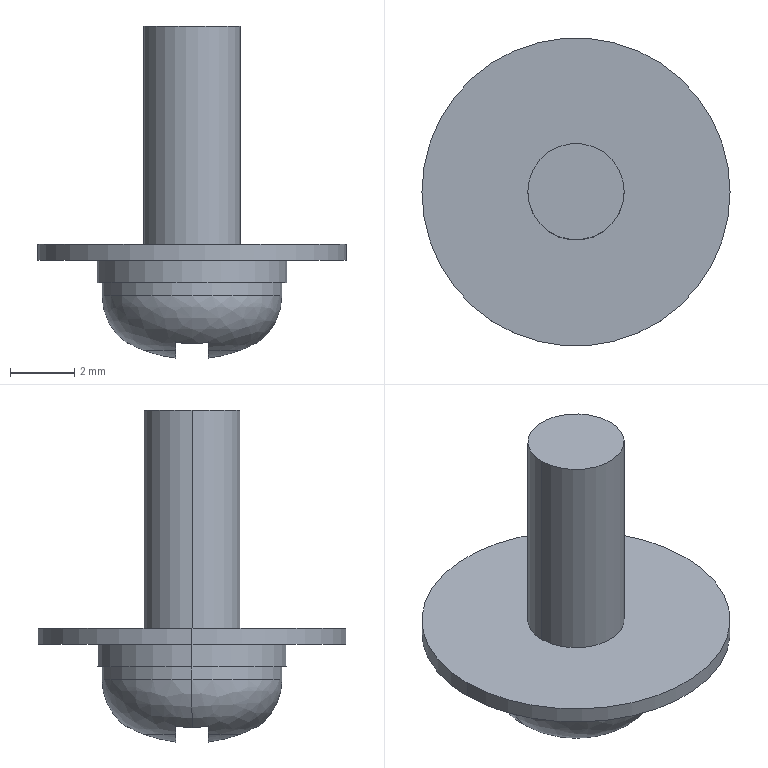Part | SolidWorks | 1 solid | 31 faces | box 9.6 x 9.6 x 10.343 mm | volume 135.072 mm3 | plane 17 | cylinder 8 | spline 6 | commonest cylinder face diameters 3 x2 5.6 x2 5.9 x2 9.6 x2
STEP:
#1=CARTESIAN_POINT('',(0.5,0.5,-1.6));
#2=VERTEX_POINT('',#1);
#3=CARTESIAN_POINT('',(0.5,2.,-1.6));
#4=VERTEX_POINT('',#3);
#5=CARTESIAN_POINT('',(0.5,2.,-1.6));
#6=DIRECTION('',(0.,1.,0.));
#7=VECTOR('',#6,1000.);
#8=LINE('',#5,#7);
#9=EDGE_CURVE('',#2,#4,#8,.T.);
#10=ORIENTED_EDGE('',*,*,#9,.T.);
#11=CARTESIAN_POINT('',(0.5,2.,-3.057));
#12=VERTEX_POINT('',#11);
#13=CARTESIAN_POINT('',(0.5,2.,-1.6));
#14=DIRECTION('',(0.,0.,-1.));
#15=VECTOR('',#14,1000.);
#16=LINE('',#13,#15);
#17=EDGE_CURVE('',#4,#12,#16,.T.);
#18=ORIENTED_EDGE('',*,*,#17,.T.);
#19=CARTESIAN_POINT('',(0.5,1.52,-3.3));
#20=VERTEX_POINT('',#19);
#21=CARTESIAN_POINT('',(0.5,2.,-3.057));
#22=CARTESIAN_POINT('',(0.5,1.853,-3.161));
#23=CARTESIAN_POINT('',(0.5,1.693,-3.242));
#24=CARTESIAN_POINT('',(0.5,1.52,-3.3));
#25=B_SPLINE_CURVE_WITH_KNOTS('',3,(#21,#22,#23,#24),.UNSPECIFIED.,.F.,.F.,(4,4),(0.,1.),.UNSPECIFIED.);
#26=EDGE_CURVE('',#12,#20,#25,.T.);
#27=ORIENTED_EDGE('',*,*,#26,.T.);
#28=CARTESIAN_POINT('',(0.5,0.5,-3.543));
#29=VERTEX_POINT('',#28);
#30=CARTESIAN_POINT('',(0.5,1.52,-3.3));
#31=CARTESIAN_POINT('',(0.5,1.19,-3.422));
#32=CARTESIAN_POINT('',(0.5,0.8497,-3.503));
#33=CARTESIAN_POINT('',(0.5,0.5,-3.543));
#34=B_SPLINE_CURVE_WITH_KNOTS('',3,(#30,#31,#32,#33),.UNSPECIFIED.,.F.,.F.,(4,4),(0.,1.),.UNSPECIFIED.);
#35=EDGE_CURVE('',#20,#29,#34,.T.);
#36=ORIENTED_EDGE('',*,*,#35,.T.);
#37=CARTESIAN_POINT('',(0.5,0.5,-1.6));
#38=DIRECTION('',(0.,0.,-1.));
#39=VECTOR('',#38,1000.);
#40=LINE('',#37,#39);
#41=EDGE_CURVE('',#2,#29,#40,.T.);
#42=ORIENTED_EDGE('',*,*,#41,.F.);
#43=EDGE_LOOP('',(#10,#18,#27,#36,#42));
#44=FACE_OUTER_BOUND('',#43,.T.);
#45=CARTESIAN_POINT('',(0.5,2.,-1.6));
#46=DIRECTION('',(-1.,0.,0.));
#47=DIRECTION('',(0.,0.,1.));
#48=AXIS2_PLACEMENT_3D('',#45,#46,#47);
#49=PLANE('',#48);
#50=ADVANCED_FACE('',(#44),#49,.T.);
#51=ORIENTED_EDGE('',*,*,#41,.T.);
#52=CARTESIAN_POINT('',(1.52,0.5,-3.3));
#53=VERTEX_POINT('',#52);
#54=CARTESIAN_POINT('',(0.,0.5,0.8167));
#55=DIRECTION('',(0.,-1.,0.));
#56=DIRECTION('',(0.,0.,1.));
#57=AXIS2_PLACEMENT_3D('',#54,#55,#56);
#58=CIRCLE('',#57,4.388);
#59=EDGE_CURVE('',#29,#53,#58,.T.);
#60=ORIENTED_EDGE('',*,*,#59,.T.);
#61=CARTESIAN_POINT('',(2.,0.5,-3.057));
#62=VERTEX_POINT('',#61);
#63=CARTESIAN_POINT('',(1.52,0.5,-3.3));
#64=CARTESIAN_POINT('',(1.691,0.5,-3.243));
#65=CARTESIAN_POINT('',(1.853,0.5,-3.161));
#66=CARTESIAN_POINT('',(2.,0.5,-3.057));
#67=B_SPLINE_CURVE_WITH_KNOTS('',3,(#63,#64,#65,#66),.UNSPECIFIED.,.F.,.F.,(4,4),(0.,0.0005389),.UNSPECIFIED.);
#68=EDGE_CURVE('',#53,#62,#67,.T.);
#69=ORIENTED_EDGE('',*,*,#68,.T.);
#70=CARTESIAN_POINT('',(2.,0.5,-1.6));
#71=VERTEX_POINT('',#70);
#72=CARTESIAN_POINT('',(2.,0.5,-1.6));
#73=DIRECTION('',(0.,0.,-1.));
#74=VECTOR('',#73,1000.);
#75=LINE('',#72,#74);
#76=EDGE_CURVE('',#71,#62,#75,.T.);
#77=ORIENTED_EDGE('',*,*,#76,.F.);
#78=CARTESIAN_POINT('',(0.5,0.5,-1.6));
#79=DIRECTION('',(-1.,0.,0.));
#80=VECTOR('',#79,1000.);
#81=LINE('',#78,#80);
#82=EDGE_CURVE('',#71,#2,#81,.T.);
#83=ORIENTED_EDGE('',*,*,#82,.T.);
#84=EDGE_LOOP('',(#51,#60,#69,#77,#83));
#85=FACE_OUTER_BOUND('',#84,.T.);
#86=CARTESIAN_POINT('',(0.5,0.5,-1.6));
#87=DIRECTION('',(0.,-1.,0.));
#88=DIRECTION('',(0.,0.,-1.));
#89=AXIS2_PLACEMENT_3D('',#86,#87,#88);
#90=PLANE('',#89);
#91=ADVANCED_FACE('',(#85),#90,.T.);
#92=CARTESIAN_POINT('',(0.5,-0.5,-1.6));
#93=VERTEX_POINT('',#92);
#94=CARTESIAN_POINT('',(2.,-0.5,-1.6));
#95=VERTEX_POINT('',#94);
#96=CARTESIAN_POINT('',(2.,-0.5,-1.6));
#97=DIRECTION('',(1.,0.,0.));
#98=VECTOR('',#97,1000.);
#99=LINE('',#96,#98);
#100=EDGE_CURVE('',#93,#95,#99,.T.);
#101=ORIENTED_EDGE('',*,*,#100,.T.);
#102=CARTESIAN_POINT('',(2.,-0.5,-3.057));
#103=VERTEX_POINT('',#102);
#104=CARTESIAN_POINT('',(2.,-0.5,-1.6));
#105=DIRECTION('',(0.,0.,1.));
#106=VECTOR('',#105,1000.);
#107=LINE('',#104,#106);
#108=EDGE_CURVE('',#103,#95,#107,.T.);
#109=ORIENTED_EDGE('',*,*,#108,.F.);
#110=CARTESIAN_POINT('',(1.52,-0.5,-3.3));
#111=VERTEX_POINT('',#110);
#112=CARTESIAN_POINT('',(2.,-0.5,-3.057));
#113=CARTESIAN_POINT('',(1.853,-0.5,-3.161));
#114=CARTESIAN_POINT('',(1.693,-0.5,-3.242));
#115=CARTESIAN_POINT('',(1.52,-0.5,-3.3));
#116=B_SPLINE_CURVE_WITH_KNOTS('',3,(#112,#113,#114,#115),.UNSPECIFIED.,.F.,.F.,(4,4),(0.,1.),.UNSPECIFIED.);
#117=EDGE_CURVE('',#103,#111,#116,.T.);
#118=ORIENTED_EDGE('',*,*,#117,.T.);
#119=CARTESIAN_POINT('',(0.5,-0.5,-3.543));
#120=VERTEX_POINT('',#119);
#121=CARTESIAN_POINT('',(0.,-0.5,0.8167));
#122=DIRECTION('',(0.,1.,0.));
#123=DIRECTION('',(0.,0.,1.));
#124=AXIS2_PLACEMENT_3D('',#121,#122,#123);
#125=CIRCLE('',#124,4.388);
#126=EDGE_CURVE('',#111,#120,#125,.T.);
#127=ORIENTED_EDGE('',*,*,#126,.T.);
#128=CARTESIAN_POINT('',(0.5,-0.5,-1.6));
#129=DIRECTION('',(0.,0.,-1.));
#130=VECTOR('',#129,1000.);
#131=LINE('',#128,#130);
#132=EDGE_CURVE('',#93,#120,#131,.T.);
#133=ORIENTED_EDGE('',*,*,#132,.F.);
#134=EDGE_LOOP('',(#101,#109,#118,#127,#133));
#135=FACE_OUTER_BOUND('',#134,.T.);
#136=CARTESIAN_POINT('',(2.,-0.5,-1.6));
#137=DIRECTION('',(0.,1.,0.));
#138=DIRECTION('',(1.,0.,0.));
#139=AXIS2_PLACEMENT_3D('',#136,#137,#138);
#140=PLANE('',#139);
#141=ADVANCED_FACE('',(#135),#140,.T.);
#142=CARTESIAN_POINT('',(-0.5,-0.5,-1.6));
#143=VERTEX_POINT('',#142);
#144=CARTESIAN_POINT('',(-0.5,-2.,-1.6));
#145=VERTEX_POINT('',#144);
#146=CARTESIAN_POINT('',(-0.5,-2.,-1.6));
#147=DIRECTION('',(0.,-1.,0.));
#148=VECTOR('',#147,1000.);
#149=LINE('',#146,#148);
#150=EDGE_CURVE('',#143,#145,#149,.T.);
#151=ORIENTED_EDGE('',*,*,#150,.T.);
#152=CARTESIAN_POINT('',(-0.5,-2.,-3.057));
#153=VERTEX_POINT('',#152);
#154=CARTESIAN_POINT('',(-0.5,-2.,-1.6));
#155=DIRECTION('',(0.,0.,-1.));
#156=VECTOR('',#155,1000.);
#157=LINE('',#154,#156);
#158=EDGE_CURVE('',#145,#153,#157,.T.);
#159=ORIENTED_EDGE('',*,*,#158,.T.);
#160=CARTESIAN_POINT('',(-0.5,-1.52,-3.3));
#161=VERTEX_POINT('',#160);
#162=CARTESIAN_POINT('',(-0.5,-2.,-3.057));
#163=CARTESIAN_POINT('',(-0.5,-1.853,-3.161));
#164=CARTESIAN_POINT('',(-0.5,-1.693,-3.242));
#165=CARTESIAN_POINT('',(-0.5,-1.52,-3.3));
#166=B_SPLINE_CURVE_WITH_KNOTS('',3,(#162,#163,#164,#165),.UNSPECIFIED.,.F.,.F.,(4,4),(0.,1.),.UNSPECIFIED.);
#167=EDGE_CURVE('',#153,#161,#166,.T.);
#168=ORIENTED_EDGE('',*,*,#167,.T.);
#169=CARTESIAN_POINT('',(-0.5,-0.5,-3.543));
#170=VERTEX_POINT('',#169);
#171=CARTESIAN_POINT('',(-0.5,-1.52,-3.3));
#172=CARTESIAN_POINT('',(-0.5,-1.19,-3.422));
#173=CARTESIAN_POINT('',(-0.5,-0.8497,-3.503));
#174=CARTESIAN_POINT('',(-0.5,-0.5,-3.543));
#175=B_SPLINE_CURVE_WITH_KNOTS('',3,(#171,#172,#173,#174),.UNSPECIFIED.,.F.,.F.,(4,4),(0.,1.),.UNSPECIFIED.);
#176=EDGE_CURVE('',#161,#170,#175,.T.);
#177=ORIENTED_EDGE('',*,*,#176,.T.);
#178=CARTESIAN_POINT('',(-0.5,-0.5,-1.6));
#179=DIRECTION('',(0.,0.,-1.));
#180=VECTOR('',#179,1000.);
#181=LINE('',#178,#180);
#182=EDGE_CURVE('',#143,#170,#181,.T.);
#183=ORIENTED_EDGE('',*,*,#182,.F.);
#184=EDGE_LOOP('',(#151,#159,#168,#177,#183));
#185=FACE_OUTER_BOUND('',#184,.T.);
#186=CARTESIAN_POINT('',(-0.5,-2.,-1.6));
#187=DIRECTION('',(1.,0.,0.));
#188=DIRECTION('',(0.,1.,0.));
#189=AXIS2_PLACEMENT_3D('',#186,#187,#188);
#190=PLANE('',#189);
#191=ADVANCED_FACE('',(#185),#190,.T.);
#192=CARTESIAN_POINT('',(2.,2.,-1.6));
#193=DIRECTION('',(0.,-1.,0.));
#194=VECTOR('',#193,1000.);
#195=LINE('',#192,#194);
#196=EDGE_CURVE('',#71,#95,#195,.T.);
#197=ORIENTED_EDGE('',*,*,#196,.F.);
#198=ORIENTED_EDGE('',*,*,#76,.T.);
#199=CARTESIAN_POINT('',(2.,0.,-3.1));
#200=VERTEX_POINT('',#199);
#201=CARTESIAN_POINT('',(2.,0.5,-3.057));
#202=CARTESIAN_POINT('',(2.,0.3381,-3.085));
#203=CARTESIAN_POINT('',(2.,0.1714,-3.1));
#204=CARTESIAN_POINT('',(2.,0.,-3.1));
#205=B_SPLINE_CURVE_WITH_KNOTS('',3,(#201,#202,#203,#204),.UNSPECIFIED.,.F.,.F.,(4,4),(0.,1.),.UNSPECIFIED.);
#206=EDGE_CURVE('',#62,#200,#205,.T.);
#207=ORIENTED_EDGE('',*,*,#206,.T.);
#208=CARTESIAN_POINT('',(2.,0.,-3.1));
#209=CARTESIAN_POINT('',(2.,-0.1714,-3.1));
#210=CARTESIAN_POINT('',(2.,-0.3381,-3.085));
#211=CARTESIAN_POINT('',(2.,-0.5,-3.057));
#212=B_SPLINE_CURVE_WITH_KNOTS('',3,(#208,#209,#210,#211),.UNSPECIFIED.,.F.,.F.,(4,4),(0.,1.),.UNSPECIFIED.);
#213=EDGE_CURVE('',#200,#103,#212,.T.);
#214=ORIENTED_EDGE('',*,*,#213,.T.);
#215=ORIENTED_EDGE('',*,*,#108,.T.);
#216=EDGE_LOOP('',(#197,#198,#207,#214,#215));
#217=FACE_OUTER_BOUND('',#216,.T.);
#218=CARTESIAN_POINT('',(2.,0.5,-1.6));
#219=DIRECTION('',(-1.,0.,0.));
#220=DIRECTION('',(0.,0.,1.));
#221=AXIS2_PLACEMENT_3D('',#218,#219,#220);
#222=PLANE('',#221);
#223=ADVANCED_FACE('',(#217),#222,.T.);
#224=ORIENTED_EDGE('',*,*,#132,.T.);
#225=CARTESIAN_POINT('',(0.5,-1.52,-3.3));
#226=VERTEX_POINT('',#225);
#227=CARTESIAN_POINT('',(0.5,-0.5,-3.543));
#228=CARTESIAN_POINT('',(0.5,-0.8497,-3.503));
#229=CARTESIAN_POINT('',(0.5,-1.19,-3.422));
#230=CARTESIAN_POINT('',(0.5,-1.52,-3.3));
#231=B_SPLINE_CURVE_WITH_KNOTS('',3,(#227,#228,#229,#230),.UNSPECIFIED.,.F.,.F.,(4,4),(0.,1.),.UNSPECIFIED.);
#232=EDGE_CURVE('',#120,#226,#231,.T.);
#233=ORIENTED_EDGE('',*,*,#232,.T.);
#234=CARTESIAN_POINT('',(0.5,-2.,-3.057));
#235=VERTEX_POINT('',#234);
#236=CARTESIAN_POINT('',(0.5,-1.52,-3.3));
#237=CARTESIAN_POINT('',(0.5,-1.691,-3.243));
#238=CARTESIAN_POINT('',(0.5,-1.853,-3.161));
#239=CARTESIAN_POINT('',(0.5,-2.,-3.057));
#240=B_SPLINE_CURVE_WITH_KNOTS('',3,(#236,#237,#238,#239),.UNSPECIFIED.,.F.,.F.,(4,4),(0.,0.0005389),.UNSPECIFIED.);
#241=EDGE_CURVE('',#226,#235,#240,.T.);
#242=ORIENTED_EDGE('',*,*,#241,.T.);
#243=CARTESIAN_POINT('',(0.5,-2.,-1.6));
#244=VERTEX_POINT('',#243);
#245=CARTESIAN_POINT('',(0.5,-2.,-1.6));
#246=DIRECTION('',(0.,0.,1.));
#247=VECTOR('',#246,1000.);
#248=LINE('',#245,#247);
#249=EDGE_CURVE('',#235,#244,#248,.T.);
#250=ORIENTED_EDGE('',*,*,#249,.T.);
#251=CARTESIAN_POINT('',(0.5,2.,-1.6));
#252=DIRECTION('',(0.,-1.,0.));
#253=VECTOR('',#252,1000.);
#254=LINE('',#251,#253);
#255=EDGE_CURVE('',#93,#244,#254,.T.);
#256=ORIENTED_EDGE('',*,*,#255,.F.);
#257=EDGE_LOOP('',(#224,#233,#242,#250,#256));
#258=FACE_OUTER_BOUND('',#257,.T.);
#259=CARTESIAN_POINT('',(0.5,-0.5,-1.6));
#260=DIRECTION('',(-1.,0.,0.));
#261=DIRECTION('',(0.,0.,1.));
#262=AXIS2_PLACEMENT_3D('',#259,#260,#261);
#263=PLANE('',#262);
#264=ADVANCED_FACE('',(#258),#263,.T.);
#265=ORIENTED_EDGE('',*,*,#182,.T.);
#266=CARTESIAN_POINT('',(-1.52,-0.5,-3.3));
#267=VERTEX_POINT('',#266);
#268=CARTESIAN_POINT('',(0.,-0.5,0.8167));
#269=DIRECTION('',(0.,1.,0.));
#270=DIRECTION('',(0.,0.,1.));
#271=AXIS2_PLACEMENT_3D('',#268,#269,#270);
#272=CIRCLE('',#271,4.388);
#273=EDGE_CURVE('',#170,#267,#272,.T.);
#274=ORIENTED_EDGE('',*,*,#273,.T.);
#275=CARTESIAN_POINT('',(-2.,-0.5,-3.057));
#276=VERTEX_POINT('',#275);
#277=CARTESIAN_POINT('',(-1.52,-0.5,-3.3));
#278=CARTESIAN_POINT('',(-1.691,-0.5,-3.243));
#279=CARTESIAN_POINT('',(-1.853,-0.5,-3.161));
#280=CARTESIAN_POINT('',(-2.,-0.5,-3.057));
#281=B_SPLINE_CURVE_WITH_KNOTS('',3,(#277,#278,#279,#280),.UNSPECIFIED.,.F.,.F.,(4,4),(0.,0.0005389),.UNSPECIFIED.);
#282=EDGE_CURVE('',#267,#276,#281,.T.);
#283=ORIENTED_EDGE('',*,*,#282,.T.);
#284=CARTESIAN_POINT('',(-2.,-0.5,-1.6));
#285=VERTEX_POINT('',#284);
#286=CARTESIAN_POINT('',(-2.,-0.5,-1.6));
#287=DIRECTION('',(0.,0.,-1.));
#288=VECTOR('',#287,1000.);
#289=LINE('',#286,#288);
#290=EDGE_CURVE('',#285,#276,#289,.T.);
#291=ORIENTED_EDGE('',*,*,#290,.F.);
#292=CARTESIAN_POINT('',(-0.5,-0.5,-1.6));
#293=DIRECTION('',(-1.,0.,0.));
#294=VECTOR('',#293,1000.);
#295=LINE('',#292,#294);
#296=EDGE_CURVE('',#143,#285,#295,.T.);
#297=ORIENTED_EDGE('',*,*,#296,.F.);
#298=EDGE_LOOP('',(#265,#274,#283,#291,#297));
#299=FACE_OUTER_BOUND('',#298,.T.);
#300=CARTESIAN_POINT('',(-0.5,-0.5,-1.6));
#301=DIRECTION('',(0.,1.,0.));
#302=DIRECTION('',(1.,0.,0.));
#303=AXIS2_PLACEMENT_3D('',#300,#301,#302);
#304=PLANE('',#303);
#305=ADVANCED_FACE('',(#299),#304,.T.);
#306=CARTESIAN_POINT('',(-0.5,0.5,-3.543));
#307=VERTEX_POINT('',#306);
#308=CARTESIAN_POINT('',(-0.5,0.5,-1.6));
#309=VERTEX_POINT('',#308);
#310=CARTESIAN_POINT('',(-0.5,0.5,-1.6));
#311=DIRECTION('',(0.,0.,1.));
#312=VECTOR('',#311,1000.);
#313=LINE('',#310,#312);
#314=EDGE_CURVE('',#307,#309,#313,.T.);
#315=ORIENTED_EDGE('',*,*,#314,.F.);
#316=CARTESIAN_POINT('',(-0.5,1.52,-3.3));
#317=VERTEX_POINT('',#316);
#318=CARTESIAN_POINT('',(-0.5,0.5,-3.543));
#319=CARTESIAN_POINT('',(-0.5,0.8497,-3.503));
#320=CARTESIAN_POINT('',(-0.5,1.19,-3.422));
#321=CARTESIAN_POINT('',(-0.5,1.52,-3.3));
#322=B_SPLINE_CURVE_WITH_KNOTS('',3,(#318,#319,#320,#321),.UNSPECIFIED.,.F.,.F.,(4,4),(0.,1.),.UNSPECIFIED.);
#323=EDGE_CURVE('',#307,#317,#322,.T.);
#324=ORIENTED_EDGE('',*,*,#323,.T.);
#325=CARTESIAN_POINT('',(-0.5,2.,-3.057));
#326=VERTEX_POINT('',#325);
#327=CARTESIAN_POINT('',(-0.5,1.52,-3.3));
#328=CARTESIAN_POINT('',(-0.5,1.691,-3.243));
#329=CARTESIAN_POINT('',(-0.5,1.853,-3.161));
#330=CARTESIAN_POINT('',(-0.5,2.,-3.057));
#331=B_SPLINE_CURVE_WITH_KNOTS('',3,(#327,#328,#329,#330),.UNSPECIFIED.,.F.,.F.,(4,4),(0.,0.0005389),.UNSPECIFIED.);
#332=EDGE_CURVE('',#317,#326,#331,.T.);
#333=ORIENTED_EDGE('',*,*,#332,.T.);
#334=CARTESIAN_POINT('',(-0.5,2.,-1.6));
#335=VERTEX_POINT('',#334);
#336=CARTESIAN_POINT('',(-0.5,2.,-1.6));
#337=DIRECTION('',(0.,0.,1.));
#338=VECTOR('',#337,1000.);
#339=LINE('',#336,#338);
#340=EDGE_CURVE('',#326,#335,#339,.T.);
#341=ORIENTED_EDGE('',*,*,#340,.T.);
#342=CARTESIAN_POINT('',(-0.5,2.,-1.6));
#343=DIRECTION('',(0.,1.,0.));
#344=VECTOR('',#343,1000.);
#345=LINE('',#342,#344);
#346=EDGE_CURVE('',#309,#335,#345,.T.);
#347=ORIENTED_EDGE('',*,*,#346,.F.);
#348=EDGE_LOOP('',(#315,#324,#333,#341,#347));
#349=FACE_OUTER_BOUND('',#348,.T.);
#350=CARTESIAN_POINT('',(-0.5,0.5,-1.6));
#351=DIRECTION('',(1.,0.,0.));
#352=DIRECTION('',(0.,1.,0.));
#353=AXIS2_PLACEMENT_3D('',#350,#351,#352);
#354=PLANE('',#353);
#355=ADVANCED_FACE('',(#349),#354,.T.);
#356=CARTESIAN_POINT('',(-2.,0.5,-1.6));
#357=VERTEX_POINT('',#356);
#358=CARTESIAN_POINT('',(-2.,2.,-1.6));
#359=DIRECTION('',(0.,1.,0.));
#360=VECTOR('',#359,1000.);
#361=LINE('',#358,#360);
#362=EDGE_CURVE('',#285,#357,#361,.T.);
#363=ORIENTED_EDGE('',*,*,#362,.F.);
#364=ORIENTED_EDGE('',*,*,#290,.T.);
#365=CARTESIAN_POINT('',(-2.,0.,-3.1));
#366=VERTEX_POINT('',#365);
#367=CARTESIAN_POINT('',(-2.,-0.5,-3.057));
#368=CARTESIAN_POINT('',(-2.,-0.3381,-3.085));
#369=CARTESIAN_POINT('',(-2.,-0.1714,-3.1));
#370=CARTESIAN_POINT('',(-2.,0.,-3.1));
#371=B_SPLINE_CURVE_WITH_KNOTS('',3,(#367,#368,#369,#370),.UNSPECIFIED.,.F.,.F.,(4,4),(0.,1.),.UNSPECIFIED.);
#372=EDGE_CURVE('',#276,#366,#371,.T.);
#373=ORIENTED_EDGE('',*,*,#372,.T.);
#374=CARTESIAN_POINT('',(-2.,0.5,-3.057));
#375=VERTEX_POINT('',#374);
#376=CARTESIAN_POINT('',(-2.,0.,-3.1));
#377=CARTESIAN_POINT('',(-2.,0.1714,-3.1));
#378=CARTESIAN_POINT('',(-2.,0.3381,-3.085));
#379=CARTESIAN_POINT('',(-2.,0.5,-3.057));
#380=B_SPLINE_CURVE_WITH_KNOTS('',3,(#376,#377,#378,#379),.UNSPECIFIED.,.F.,.F.,(4,4),(0.,1.),.UNSPECIFIED.);
#381=EDGE_CURVE('',#366,#375,#380,.T.);
#382=ORIENTED_EDGE('',*,*,#381,.T.);
#383=CARTESIAN_POINT('',(-2.,0.5,-1.6));
#384=DIRECTION('',(0.,0.,-1.));
#385=VECTOR('',#384,1000.);
#386=LINE('',#383,#385);
#387=EDGE_CURVE('',#357,#375,#386,.T.);
#388=ORIENTED_EDGE('',*,*,#387,.F.);
#389=EDGE_LOOP('',(#363,#364,#373,#382,#388));
#390=FACE_OUTER_BOUND('',#389,.T.);
#391=CARTESIAN_POINT('',(-2.,-0.5,-1.6));
#392=DIRECTION('',(1.,0.,0.));
#393=DIRECTION('',(0.,1.,0.));
#394=AXIS2_PLACEMENT_3D('',#391,#392,#393);
#395=PLANE('',#394);
#396=ADVANCED_FACE('',(#390),#395,.T.);
#397=ORIENTED_EDGE('',*,*,#362,.T.);
#398=CARTESIAN_POINT('',(-2.,0.5,-1.6));
#399=DIRECTION('',(-1.,0.,0.));
#400=VECTOR('',#399,1000.);
#401=LINE('',#398,#400);
#402=EDGE_CURVE('',#309,#357,#401,.T.);
#403=ORIENTED_EDGE('',*,*,#402,.F.);
#404=ORIENTED_EDGE('',*,*,#346,.T.);
#405=CARTESIAN_POINT('',(-0.5,2.,-1.6));
#406=DIRECTION('',(-1.,0.,0.));
#407=VECTOR('',#406,1000.);
#408=LINE('',#405,#407);
#409=EDGE_CURVE('',#4,#335,#408,.T.);
#410=ORIENTED_EDGE('',*,*,#409,.F.);
#411=ORIENTED_EDGE('',*,*,#9,.F.);
#412=ORIENTED_EDGE('',*,*,#82,.F.);
#413=ORIENTED_EDGE('',*,*,#196,.T.);
#414=ORIENTED_EDGE('',*,*,#100,.F.);
#415=ORIENTED_EDGE('',*,*,#255,.T.);
#416=CARTESIAN_POINT('',(0.5,-2.,-1.6));
#417=DIRECTION('',(1.,0.,0.));
#418=VECTOR('',#417,1000.);
#419=LINE('',#416,#418);
#420=EDGE_CURVE('',#145,#244,#419,.T.);
#421=ORIENTED_EDGE('',*,*,#420,.F.);
#422=ORIENTED_EDGE('',*,*,#150,.F.);
#423=ORIENTED_EDGE('',*,*,#296,.T.);
#424=EDGE_LOOP('',(#397,#403,#404,#410,#411,#412,#413,#414,#415,#421,#422,#423));
#425=FACE_OUTER_BOUND('',#424,.T.);
#426=CARTESIAN_POINT('',(-0.5,2.,-1.6));
#427=DIRECTION('',(0.,0.,-1.));
#428=DIRECTION('',(0.,-1.,0.));
#429=AXIS2_PLACEMENT_3D('',#426,#427,#428);
#430=PLANE('',#429);
#431=ADVANCED_FACE('',(#425),#430,.T.);
#432=ORIENTED_EDGE('',*,*,#402,.T.);
#433=ORIENTED_EDGE('',*,*,#387,.T.);
#434=CARTESIAN_POINT('',(-1.52,0.5,-3.3));
#435=VERTEX_POINT('',#434);
#436=CARTESIAN_POINT('',(-2.,0.5,-3.057));
#437=CARTESIAN_POINT('',(-1.853,0.5,-3.161));
#438=CARTESIAN_POINT('',(-1.693,0.5,-3.242));
#439=CARTESIAN_POINT('',(-1.52,0.5,-3.3));
#440=B_SPLINE_CURVE_WITH_KNOTS('',3,(#436,#437,#438,#439),.UNSPECIFIED.,.F.,.F.,(4,4),(0.,1.),.UNSPECIFIED.);
#441=EDGE_CURVE('',#375,#435,#440,.T.);
#442=ORIENTED_EDGE('',*,*,#441,.T.);
#443=CARTESIAN_POINT('',(0.,0.5,0.8167));
#444=DIRECTION('',(0.,1.,0.));
#445=DIRECTION('',(0.,0.,1.));
#446=AXIS2_PLACEMENT_3D('',#443,#444,#445);
#447=CIRCLE('',#446,4.388);
#448=EDGE_CURVE('',#307,#435,#447,.T.);
#449=ORIENTED_EDGE('',*,*,#448,.F.);
#450=ORIENTED_EDGE('',*,*,#314,.T.);
#451=EDGE_LOOP('',(#432,#433,#442,#449,#450));
#452=FACE_OUTER_BOUND('',#451,.T.);
#453=CARTESIAN_POINT('',(-2.,0.5,-1.6));
#454=DIRECTION('',(0.,-1.,0.));
#455=DIRECTION('',(0.,0.,-1.));
#456=AXIS2_PLACEMENT_3D('',#453,#454,#455);
#457=PLANE('',#456);
#458=ADVANCED_FACE('',(#452),#457,.T.);
#459=ORIENTED_EDGE('',*,*,#176,.F.);
#460=CARTESIAN_POINT('',(0.,0.,-3.3));
#461=DIRECTION('',(0.,0.,1.));
#462=DIRECTION('',(1.,0.,0.));
#463=AXIS2_PLACEMENT_3D('',#460,#461,#462);
#464=CIRCLE('',#463,1.6);
#465=EDGE_CURVE('',#267,#161,#464,.T.);
#466=ORIENTED_EDGE('',*,*,#465,.F.);
#467=ORIENTED_EDGE('',*,*,#273,.F.);
#468=EDGE_LOOP('',(#459,#466,#467));
#469=FACE_OUTER_BOUND('',#468,.T.);
#470=CARTESIAN_POINT('',(-0.4937,-0.5,-3.544));
#471=CARTESIAN_POINT('',(-0.8469,-0.5,-3.504));
#472=CARTESIAN_POINT('',(-1.193,-0.5,-3.421));
#473=CARTESIAN_POINT('',(-1.526,-0.5,-3.298));
#474=CARTESIAN_POINT('',(-0.4892,-0.8509,-3.504));
#475=CARTESIAN_POINT('',(-0.8392,-0.8509,-3.464));
#476=CARTESIAN_POINT('',(-1.182,-0.8509,-3.383));
#477=CARTESIAN_POINT('',(-1.512,-0.8509,-3.26));
#478=CARTESIAN_POINT('',(-0.4801,-1.194,-3.423));
#479=CARTESIAN_POINT('',(-0.8234,-1.194,-3.384));
#480=CARTESIAN_POINT('',(-1.16,-1.194,-3.304));
#481=CARTESIAN_POINT('',(-1.484,-1.194,-3.184));
#482=CARTESIAN_POINT('',(-0.4663,-1.526,-3.302));
#483=CARTESIAN_POINT('',(-0.7999,-1.526,-3.264));
#484=CARTESIAN_POINT('',(-1.126,-1.526,-3.186));
#485=CARTESIAN_POINT('',(-1.441,-1.526,-3.069));
#486=(BOUNDED_SURFACE()B_SPLINE_SURFACE(3,3,((#470,#471,#472,#473),(#474,#475,#476,#477),(#478,#479,#480,#481),(#482,#483,#484,#485)),.UNSPECIFIED.,.F.,.F.,.F.)B_SPLINE_SURFACE_WITH_KNOTS((4,4),(4,4),(0.,1.),(0.,1.),.UNSPECIFIED.)GEOMETRIC_REPRESENTATION_ITEM()RATIONAL_B_SPLINE_SURFACE(((1.,0.9951,0.9951,1.),(0.9952,0.9904,0.9904,0.9952),(0.9952,0.9904,0.9904,0.9952),(1.,0.9951,0.9951,1.)))REPRESENTATION_ITEM('')SURFACE());
#487=ADVANCED_FACE('',(#469),#486,.T.);
#488=ORIENTED_EDGE('',*,*,#420,.T.);
#489=ORIENTED_EDGE('',*,*,#249,.F.);
#490=CARTESIAN_POINT('',(-0.5,-2.,-3.057));
#491=CARTESIAN_POINT('',(-0.3327,-2.,-3.086));
#492=CARTESIAN_POINT('',(-0.1684,-2.,-3.1));
#493=CARTESIAN_POINT('',(0.1684,-2.,-3.1));
#494=CARTESIAN_POINT('',(0.3327,-2.,-3.086));
#495=CARTESIAN_POINT('',(0.5,-2.,-3.057));
#496=B_SPLINE_CURVE_WITH_KNOTS('',3,(#490,#491,#492,#493,#494,#495),.UNSPECIFIED.,.F.,.F.,(4,2,4),(0.,0.5,1.),.UNSPECIFIED.);
#497=EDGE_CURVE('',#153,#235,#496,.T.);
#498=ORIENTED_EDGE('',*,*,#497,.F.);
#499=ORIENTED_EDGE('',*,*,#158,.F.);
#500=EDGE_LOOP('',(#488,#489,#498,#499));
#501=FACE_OUTER_BOUND('',#500,.T.);
#502=CARTESIAN_POINT('',(0.5,-2.,-1.6));
#503=DIRECTION('',(0.,1.,0.));
#504=DIRECTION('',(1.,0.,0.));
#505=AXIS2_PLACEMENT_3D('',#502,#503,#504);
#506=PLANE('',#505);
#507=ADVANCED_FACE('',(#501),#506,.T.);
#508=ORIENTED_EDGE('',*,*,#126,.F.);
#509=CARTESIAN_POINT('',(0.,0.,-3.3));
#510=DIRECTION('',(0.,0.,1.));
#511=DIRECTION('',(1.,0.,0.));
#512=AXIS2_PLACEMENT_3D('',#509,#510,#511);
#513=CIRCLE('',#512,1.6);
#514=EDGE_CURVE('',#226,#111,#513,.T.);
#515=ORIENTED_EDGE('',*,*,#514,.F.);
#516=ORIENTED_EDGE('',*,*,#232,.F.);
#517=EDGE_LOOP('',(#508,#515,#516));
#518=FACE_OUTER_BOUND('',#517,.T.);
#519=CARTESIAN_POINT('',(1.526,-0.5,-3.298));
#520=CARTESIAN_POINT('',(1.193,-0.5,-3.421));
#521=CARTESIAN_POINT('',(0.8469,-0.5,-3.504));
#522=CARTESIAN_POINT('',(0.4937,-0.5,-3.544));
#523=CARTESIAN_POINT('',(1.512,-0.8509,-3.26));
#524=CARTESIAN_POINT('',(1.182,-0.8509,-3.383));
#525=CARTESIAN_POINT('',(0.8392,-0.8509,-3.464));
#526=CARTESIAN_POINT('',(0.4892,-0.8509,-3.504));
#527=CARTESIAN_POINT('',(1.484,-1.194,-3.184));
#528=CARTESIAN_POINT('',(1.16,-1.194,-3.304));
#529=CARTESIAN_POINT('',(0.8234,-1.194,-3.384));
#530=CARTESIAN_POINT('',(0.4801,-1.194,-3.423));
#531=CARTESIAN_POINT('',(1.441,-1.526,-3.069));
#532=CARTESIAN_POINT('',(1.126,-1.526,-3.186));
#533=CARTESIAN_POINT('',(0.7999,-1.526,-3.264));
#534=CARTESIAN_POINT('',(0.4663,-1.526,-3.302));
#535=(BOUNDED_SURFACE()B_SPLINE_SURFACE(3,3,((#519,#520,#521,#522),(#523,#524,#525,#526),(#527,#528,#529,#530),(#531,#532,#533,#534)),.UNSPECIFIED.,.F.,.F.,.T.)B_SPLINE_SURFACE_WITH_KNOTS((4,4),(4,4),(0.,1.),(0.,1.),.UNSPECIFIED.)GEOMETRIC_REPRESENTATION_ITEM()RATIONAL_B_SPLINE_SURFACE(((1.,0.9951,0.9951,1.),(0.9952,0.9904,0.9904,0.9952),(0.9952,0.9904,0.9904,0.9952),(1.,0.9951,0.9951,1.)))REPRESENTATION_ITEM('')SURFACE());
#536=ADVANCED_FACE('',(#518),#535,.T.);
#537=ORIENTED_EDGE('',*,*,#35,.F.);
#538=CARTESIAN_POINT('',(0.,0.,-3.3));
#539=DIRECTION('',(0.,0.,1.));
#540=DIRECTION('',(1.,0.,0.));
#541=AXIS2_PLACEMENT_3D('',#538,#539,#540);
#542=CIRCLE('',#541,1.6);
#543=EDGE_CURVE('',#53,#20,#542,.T.);
#544=ORIENTED_EDGE('',*,*,#543,.F.);
#545=ORIENTED_EDGE('',*,*,#59,.F.);
#546=EDGE_LOOP('',(#537,#544,#545));
#547=FACE_OUTER_BOUND('',#546,.T.);
#548=CARTESIAN_POINT('',(1.441,1.526,-3.069));
#549=CARTESIAN_POINT('',(1.126,1.526,-3.186));
#550=CARTESIAN_POINT('',(0.7999,1.526,-3.264));
#551=CARTESIAN_POINT('',(0.4663,1.526,-3.302));
#552=CARTESIAN_POINT('',(1.484,1.194,-3.184));
#553=CARTESIAN_POINT('',(1.16,1.194,-3.304));
#554=CARTESIAN_POINT('',(0.8234,1.194,-3.384));
#555=CARTESIAN_POINT('',(0.4801,1.194,-3.423));
#556=CARTESIAN_POINT('',(1.512,0.8509,-3.26));
#557=CARTESIAN_POINT('',(1.182,0.8509,-3.383));
#558=CARTESIAN_POINT('',(0.8392,0.8509,-3.464));
#559=CARTESIAN_POINT('',(0.4892,0.8509,-3.504));
#560=CARTESIAN_POINT('',(1.526,0.5,-3.298));
#561=CARTESIAN_POINT('',(1.193,0.5,-3.421));
#562=CARTESIAN_POINT('',(0.8469,0.5,-3.504));
#563=CARTESIAN_POINT('',(0.4937,0.5,-3.544));
#564=(BOUNDED_SURFACE()B_SPLINE_SURFACE(3,3,((#548,#549,#550,#551),(#552,#553,#554,#555),(#556,#557,#558,#559),(#560,#561,#562,#563)),.UNSPECIFIED.,.F.,.F.,.T.)B_SPLINE_SURFACE_WITH_KNOTS((4,4),(4,4),(0.,1.),(0.,1.),.UNSPECIFIED.)GEOMETRIC_REPRESENTATION_ITEM()RATIONAL_B_SPLINE_SURFACE(((1.,0.9951,0.9951,1.),(0.9952,0.9904,0.9904,0.9952),(0.9952,0.9904,0.9904,0.9952),(1.,0.9951,0.9951,1.)))REPRESENTATION_ITEM('')SURFACE());
#565=ADVANCED_FACE('',(#547),#564,.T.);
#566=ORIENTED_EDGE('',*,*,#409,.T.);
#567=ORIENTED_EDGE('',*,*,#340,.F.);
#568=CARTESIAN_POINT('',(0.5,2.,-3.057));
#569=CARTESIAN_POINT('',(0.3327,2.,-3.086));
#570=CARTESIAN_POINT('',(0.1684,2.,-3.1));
#571=CARTESIAN_POINT('',(-0.1684,2.,-3.1));
#572=CARTESIAN_POINT('',(-0.3327,2.,-3.086));
#573=CARTESIAN_POINT('',(-0.5,2.,-3.057));
#574=B_SPLINE_CURVE_WITH_KNOTS('',3,(#568,#569,#570,#571,#572,#573),.UNSPECIFIED.,.F.,.F.,(4,2,4),(0.,0.5,1.),.UNSPECIFIED.);
#575=EDGE_CURVE('',#12,#326,#574,.T.);
#576=ORIENTED_EDGE('',*,*,#575,.F.);
#577=ORIENTED_EDGE('',*,*,#17,.F.);
#578=EDGE_LOOP('',(#566,#567,#576,#577));
#579=FACE_OUTER_BOUND('',#578,.T.);
#580=CARTESIAN_POINT('',(-0.5,2.,-1.6));
#581=DIRECTION('',(0.,-1.,0.));
#582=DIRECTION('',(0.,0.,-1.));
#583=AXIS2_PLACEMENT_3D('',#580,#581,#582);
#584=PLANE('',#583);
#585=ADVANCED_FACE('',(#579),#584,.T.);
#586=ORIENTED_EDGE('',*,*,#448,.T.);
#587=CARTESIAN_POINT('',(0.,0.,-3.3));
#588=DIRECTION('',(0.,0.,1.));
#589=DIRECTION('',(1.,0.,0.));
#590=AXIS2_PLACEMENT_3D('',#587,#588,#589);
#591=CIRCLE('',#590,1.6);
#592=EDGE_CURVE('',#317,#435,#591,.T.);
#593=ORIENTED_EDGE('',*,*,#592,.F.);
#594=ORIENTED_EDGE('',*,*,#323,.F.);
#595=EDGE_LOOP('',(#586,#593,#594));
#596=FACE_OUTER_BOUND('',#595,.T.);
#597=CARTESIAN_POINT('',(-0.4663,1.526,-3.302));
#598=CARTESIAN_POINT('',(-0.7999,1.526,-3.264));
#599=CARTESIAN_POINT('',(-1.126,1.526,-3.186));
#600=CARTESIAN_POINT('',(-1.441,1.526,-3.069));
#601=CARTESIAN_POINT('',(-0.4801,1.194,-3.423));
#602=CARTESIAN_POINT('',(-0.8234,1.194,-3.384));
#603=CARTESIAN_POINT('',(-1.16,1.194,-3.304));
#604=CARTESIAN_POINT('',(-1.484,1.194,-3.184));
#605=CARTESIAN_POINT('',(-0.4892,0.8509,-3.504));
#606=CARTESIAN_POINT('',(-0.8392,0.8509,-3.464));
#607=CARTESIAN_POINT('',(-1.182,0.8509,-3.383));
#608=CARTESIAN_POINT('',(-1.512,0.8509,-3.26));
#609=CARTESIAN_POINT('',(-0.4937,0.5,-3.544));
#610=CARTESIAN_POINT('',(-0.8469,0.5,-3.504));
#611=CARTESIAN_POINT('',(-1.193,0.5,-3.421));
#612=CARTESIAN_POINT('',(-1.526,0.5,-3.298));
#613=(BOUNDED_SURFACE()B_SPLINE_SURFACE(3,3,((#597,#598,#599,#600),(#601,#602,#603,#604),(#605,#606,#607,#608),(#609,#610,#611,#612)),.UNSPECIFIED.,.F.,.F.,.T.)B_SPLINE_SURFACE_WITH_KNOTS((4,4),(4,4),(0.,1.),(0.,1.),.UNSPECIFIED.)GEOMETRIC_REPRESENTATION_ITEM()RATIONAL_B_SPLINE_SURFACE(((1.,0.9951,0.9951,1.),(0.9952,0.9904,0.9904,0.9952),(0.9952,0.9904,0.9904,0.9952),(1.,0.9951,0.9951,1.)))REPRESENTATION_ITEM('')SURFACE());
#614=ADVANCED_FACE('',(#596),#613,.T.);
#615=CARTESIAN_POINT('',(-2.8,0.,-1.603));
#616=VERTEX_POINT('',#615);
#617=CARTESIAN_POINT('',(-1.,0.,-1.603));
#618=DIRECTION('',(0.,-1.,0.));
#619=DIRECTION('',(-1.,0.,0.));
#620=AXIS2_PLACEMENT_3D('',#617,#618,#619);
#621=CIRCLE('',#620,1.8);
#622=EDGE_CURVE('',#616,#366,#621,.T.);
#623=ORIENTED_EDGE('',*,*,#622,.F.);
#624=CARTESIAN_POINT('',(2.8,0.,-1.603));
#625=VERTEX_POINT('',#624);
#626=CARTESIAN_POINT('',(0.,0.,-1.603));
#627=DIRECTION('',(0.,0.,1.));
#628=DIRECTION('',(1.,0.,0.));
#629=AXIS2_PLACEMENT_3D('',#626,#627,#628);
#630=CIRCLE('',#629,2.8);
#631=EDGE_CURVE('',#625,#616,#630,.T.);
#632=ORIENTED_EDGE('',*,*,#631,.F.);
#633=CARTESIAN_POINT('',(1.,0.,-1.603));
#634=DIRECTION('',(0.,1.,0.));
#635=DIRECTION('',(1.,0.,0.));
#636=AXIS2_PLACEMENT_3D('',#633,#634,#635);
#637=CIRCLE('',#636,1.8);
#638=EDGE_CURVE('',#625,#200,#637,.T.);
#639=ORIENTED_EDGE('',*,*,#638,.T.);
#640=ORIENTED_EDGE('',*,*,#206,.F.);
#641=ORIENTED_EDGE('',*,*,#68,.F.);
#642=ORIENTED_EDGE('',*,*,#543,.T.);
#643=ORIENTED_EDGE('',*,*,#26,.F.);
#644=ORIENTED_EDGE('',*,*,#575,.T.);
#645=ORIENTED_EDGE('',*,*,#332,.F.);
#646=ORIENTED_EDGE('',*,*,#592,.T.);
#647=ORIENTED_EDGE('',*,*,#441,.F.);
#648=ORIENTED_EDGE('',*,*,#381,.F.);
#649=EDGE_LOOP('',(#623,#632,#639,#640,#641,#642,#643,#644,#645,#646,#647,#648));
#650=FACE_OUTER_BOUND('',#649,.T.);
#651=CARTESIAN_POINT('',(2.8,0.,-1.603));
#652=CARTESIAN_POINT('',(2.8,5.6,-1.603));
#653=CARTESIAN_POINT('',(-2.8,5.6,-1.603));
#654=CARTESIAN_POINT('',(-2.8,0.,-1.603));
#655=CARTESIAN_POINT('',(2.8,0.,-2.392));
#656=CARTESIAN_POINT('',(2.8,5.6,-2.392));
#657=CARTESIAN_POINT('',(-2.8,5.6,-2.392));
#658=CARTESIAN_POINT('',(-2.8,0.,-2.392));
#659=CARTESIAN_POINT('',(2.344,0.,-3.037));
#660=CARTESIAN_POINT('',(2.344,4.689,-3.037));
#661=CARTESIAN_POINT('',(-2.344,4.689,-3.037));
#662=CARTESIAN_POINT('',(-2.344,0.,-3.037));
#663=CARTESIAN_POINT('',(1.6,0.,-3.3));
#664=CARTESIAN_POINT('',(1.6,3.2,-3.3));
#665=CARTESIAN_POINT('',(-1.6,3.2,-3.3));
#666=CARTESIAN_POINT('',(-1.6,0.,-3.3));
#667=(BOUNDED_SURFACE()B_SPLINE_SURFACE(3,3,((#651,#652,#653,#654),(#655,#656,#657,#658),(#659,#660,#661,#662),(#663,#664,#665,#666)),.UNSPECIFIED.,.F.,.F.,.F.)B_SPLINE_SURFACE_WITH_KNOTS((4,4),(4,4),(0.,1.),(0.,1.),.UNSPECIFIED.)GEOMETRIC_REPRESENTATION_ITEM()RATIONAL_B_SPLINE_SURFACE(((1.,0.3333,0.3333,1.),(0.8777,0.2926,0.2926,0.8777),(0.8777,0.2926,0.2926,0.8777),(1.,0.3333,0.3333,1.)))REPRESENTATION_ITEM('')SURFACE());
#668=ADVANCED_FACE('',(#650),#667,.T.);
#669=CARTESIAN_POINT('',(-2.8,0.,-1.2));
#670=VERTEX_POINT('',#669);
#671=CARTESIAN_POINT('',(-2.8,0.,25.466));
#672=DIRECTION('',(0.,0.,1.));
#673=VECTOR('',#672,1000.);
#674=LINE('',#671,#673);
#675=EDGE_CURVE('',#616,#670,#674,.T.);
#676=ORIENTED_EDGE('',*,*,#675,.F.);
#677=CARTESIAN_POINT('',(0.,0.,-1.603));
#678=DIRECTION('',(0.,0.,1.));
#679=DIRECTION('',(1.,0.,0.));
#680=AXIS2_PLACEMENT_3D('',#677,#678,#679);
#681=CIRCLE('',#680,2.8);
#682=EDGE_CURVE('',#616,#625,#681,.T.);
#683=ORIENTED_EDGE('',*,*,#682,.T.);
#684=CARTESIAN_POINT('',(2.8,0.,-1.2));
#685=VERTEX_POINT('',#684);
#686=CARTESIAN_POINT('',(2.8,0.,25.466));
#687=DIRECTION('',(0.,0.,1.));
#688=VECTOR('',#687,1000.);
#689=LINE('',#686,#688);
#690=EDGE_CURVE('',#625,#685,#689,.T.);
#691=ORIENTED_EDGE('',*,*,#690,.T.);
#692=CARTESIAN_POINT('',(0.,0.,-1.2));
#693=DIRECTION('',(0.,0.,-1.));
#694=DIRECTION('',(1.,0.,0.));
#695=AXIS2_PLACEMENT_3D('',#692,#693,#694);
#696=CIRCLE('',#695,2.8);
#697=EDGE_CURVE('',#685,#670,#696,.T.);
#698=ORIENTED_EDGE('',*,*,#697,.T.);
#699=EDGE_LOOP('',(#676,#683,#691,#698));
#700=FACE_OUTER_BOUND('',#699,.T.);
#701=CARTESIAN_POINT('',(0.,0.,25.466));
#702=DIRECTION('',(0.,0.,1.));
#703=DIRECTION('',(1.,0.,0.));
#704=AXIS2_PLACEMENT_3D('',#701,#702,#703);
#705=CYLINDRICAL_SURFACE('',#704,2.8);
#706=ADVANCED_FACE('',(#700),#705,.T.);
#707=ORIENTED_EDGE('',*,*,#697,.F.);
#708=CARTESIAN_POINT('',(0.,0.,-1.2));
#709=DIRECTION('',(0.,0.,-1.));
#710=DIRECTION('',(1.,0.,0.));
#711=AXIS2_PLACEMENT_3D('',#708,#709,#710);
#712=CIRCLE('',#711,2.8);
#713=EDGE_CURVE('',#670,#685,#712,.T.);
#714=ORIENTED_EDGE('',*,*,#713,.F.);
#715=EDGE_LOOP('',(#707,#714));
#716=FACE_BOUND('',#715,.T.);
#717=CARTESIAN_POINT('',(2.95,0.,-1.2));
#718=VERTEX_POINT('',#717);
#719=CARTESIAN_POINT('',(-2.95,0.,-1.2));
#720=VERTEX_POINT('',#719);
#721=CARTESIAN_POINT('',(0.,0.,-1.2));
#722=DIRECTION('',(0.,0.,1.));
#723=DIRECTION('',(1.,0.,0.));
#724=AXIS2_PLACEMENT_3D('',#721,#722,#723);
#725=CIRCLE('',#724,2.95);
#726=EDGE_CURVE('',#718,#720,#725,.T.);
#727=ORIENTED_EDGE('',*,*,#726,.F.);
#728=CARTESIAN_POINT('',(0.,0.,-1.2));
#729=DIRECTION('',(0.,0.,1.));
#730=DIRECTION('',(1.,0.,0.));
#731=AXIS2_PLACEMENT_3D('',#728,#729,#730);
#732=CIRCLE('',#731,2.95);
#733=EDGE_CURVE('',#720,#718,#732,.T.);
#734=ORIENTED_EDGE('',*,*,#733,.F.);
#735=EDGE_LOOP('',(#727,#734));
#736=FACE_OUTER_BOUND('',#735,.T.);
#737=CARTESIAN_POINT('',(0.,2.8,-1.2));
#738=DIRECTION('',(0.,0.,1.));
#739=DIRECTION('',(1.,0.,0.));
#740=AXIS2_PLACEMENT_3D('',#737,#738,#739);
#741=PLANE('',#740);
#742=ADVANCED_FACE('',(#716,#736),#741,.F.);
#743=CARTESIAN_POINT('',(-2.95,0.,-0.5));
#744=VERTEX_POINT('',#743);
#745=CARTESIAN_POINT('',(-2.95,0.,25.466));
#746=DIRECTION('',(0.,0.,1.));
#747=VECTOR('',#746,1000.);
#748=LINE('',#745,#747);
#749=EDGE_CURVE('',#720,#744,#748,.T.);
#750=ORIENTED_EDGE('',*,*,#749,.F.);
#751=ORIENTED_EDGE('',*,*,#733,.T.);
#752=CARTESIAN_POINT('',(2.95,0.,-0.5));
#753=VERTEX_POINT('',#752);
#754=CARTESIAN_POINT('',(2.95,0.,25.466));
#755=DIRECTION('',(0.,0.,1.));
#756=VECTOR('',#755,1000.);
#757=LINE('',#754,#756);
#758=EDGE_CURVE('',#718,#753,#757,.T.);
#759=ORIENTED_EDGE('',*,*,#758,.T.);
#760=CARTESIAN_POINT('',(0.,0.,-0.5));
#761=DIRECTION('',(0.,0.,-1.));
#762=DIRECTION('',(1.,0.,0.));
#763=AXIS2_PLACEMENT_3D('',#760,#761,#762);
#764=CIRCLE('',#763,2.95);
#765=EDGE_CURVE('',#753,#744,#764,.T.);
#766=ORIENTED_EDGE('',*,*,#765,.T.);
#767=EDGE_LOOP('',(#750,#751,#759,#766));
#768=FACE_OUTER_BOUND('',#767,.T.);
#769=CARTESIAN_POINT('',(0.,0.,25.466));
#770=DIRECTION('',(0.,0.,1.));
#771=DIRECTION('',(1.,0.,0.));
#772=AXIS2_PLACEMENT_3D('',#769,#770,#771);
#773=CYLINDRICAL_SURFACE('',#772,2.95);
#774=ADVANCED_FACE('',(#768),#773,.T.);
#775=CARTESIAN_POINT('',(1.5,0.,6.8));
#776=VERTEX_POINT('',#775);
#777=CARTESIAN_POINT('',(-1.5,0.,6.8));
#778=VERTEX_POINT('',#777);
#779=CARTESIAN_POINT('',(0.,0.,6.8));
#780=DIRECTION('',(0.,0.,-1.));
#781=DIRECTION('',(1.,0.,0.));
#782=AXIS2_PLACEMENT_3D('',#779,#780,#781);
#783=CIRCLE('',#782,1.5);
#784=EDGE_CURVE('',#776,#778,#783,.T.);
#785=ORIENTED_EDGE('',*,*,#784,.F.);
#786=CARTESIAN_POINT('',(0.,0.,6.8));
#787=DIRECTION('',(0.,0.,-1.));
#788=DIRECTION('',(1.,0.,0.));
#789=AXIS2_PLACEMENT_3D('',#786,#787,#788);
#790=CIRCLE('',#789,1.5);
#791=EDGE_CURVE('',#778,#776,#790,.T.);
#792=ORIENTED_EDGE('',*,*,#791,.F.);
#793=EDGE_LOOP('',(#785,#792));
#794=FACE_OUTER_BOUND('',#793,.T.);
#795=CARTESIAN_POINT('',(0.,1.5,6.8));
#796=DIRECTION('',(0.,0.,-1.));
#797=DIRECTION('',(0.,-1.,0.));
#798=AXIS2_PLACEMENT_3D('',#795,#796,#797);
#799=PLANE('',#798);
#800=ADVANCED_FACE('',(#794),#799,.F.);
#801=ORIENTED_EDGE('',*,*,#765,.F.);
#802=CARTESIAN_POINT('',(0.,0.,-0.5));
#803=DIRECTION('',(0.,0.,-1.));
#804=DIRECTION('',(1.,0.,0.));
#805=AXIS2_PLACEMENT_3D('',#802,#803,#804);
#806=CIRCLE('',#805,2.95);
#807=EDGE_CURVE('',#744,#753,#806,.T.);
#808=ORIENTED_EDGE('',*,*,#807,.F.);
#809=EDGE_LOOP('',(#801,#808));
#810=FACE_BOUND('',#809,.T.);
#811=CARTESIAN_POINT('',(4.8,0.,-0.5));
#812=VERTEX_POINT('',#811);
#813=CARTESIAN_POINT('',(-4.8,0.,-0.5));
#814=VERTEX_POINT('',#813);
#815=CARTESIAN_POINT('',(0.,0.,-0.5));
#816=DIRECTION('',(0.,0.,1.));
#817=DIRECTION('',(1.,0.,0.));
#818=AXIS2_PLACEMENT_3D('',#815,#816,#817);
#819=CIRCLE('',#818,4.8);
#820=EDGE_CURVE('',#812,#814,#819,.T.);
#821=ORIENTED_EDGE('',*,*,#820,.F.);
#822=CARTESIAN_POINT('',(0.,0.,-0.5));
#823=DIRECTION('',(0.,0.,1.));
#824=DIRECTION('',(1.,0.,0.));
#825=AXIS2_PLACEMENT_3D('',#822,#823,#824);
#826=CIRCLE('',#825,4.8);
#827=EDGE_CURVE('',#814,#812,#826,.T.);
#828=ORIENTED_EDGE('',*,*,#827,.F.);
#829=EDGE_LOOP('',(#821,#828));
#830=FACE_OUTER_BOUND('',#829,.T.);
#831=CARTESIAN_POINT('',(0.,2.95,-0.5));
#832=DIRECTION('',(0.,0.,1.));
#833=DIRECTION('',(1.,0.,0.));
#834=AXIS2_PLACEMENT_3D('',#831,#832,#833);
#835=PLANE('',#834);
#836=ADVANCED_FACE('',(#810,#830),#835,.F.);
#837=CARTESIAN_POINT('',(-1.5,0.,0.));
#838=VERTEX_POINT('',#837);
#839=CARTESIAN_POINT('',(-1.5,0.,25.466));
#840=DIRECTION('',(0.,0.,1.));
#841=VECTOR('',#840,1000.);
#842=LINE('',#839,#841);
#843=EDGE_CURVE('',#838,#778,#842,.T.);
#844=ORIENTED_EDGE('',*,*,#843,.F.);
#845=CARTESIAN_POINT('',(1.5,0.,0.));
#846=VERTEX_POINT('',#845);
#847=CARTESIAN_POINT('',(0.,0.,0.));
#848=DIRECTION('',(0.,0.,1.));
#849=DIRECTION('',(1.,0.,0.));
#850=AXIS2_PLACEMENT_3D('',#847,#848,#849);
#851=CIRCLE('',#850,1.5);
#852=EDGE_CURVE('',#838,#846,#851,.T.);
#853=ORIENTED_EDGE('',*,*,#852,.T.);
#854=CARTESIAN_POINT('',(1.5,0.,25.466));
#855=DIRECTION('',(0.,0.,1.));
#856=VECTOR('',#855,1000.);
#857=LINE('',#854,#856);
#858=EDGE_CURVE('',#846,#776,#857,.T.);
#859=ORIENTED_EDGE('',*,*,#858,.T.);
#860=ORIENTED_EDGE('',*,*,#784,.T.);
#861=EDGE_LOOP('',(#844,#853,#859,#860));
#862=FACE_OUTER_BOUND('',#861,.T.);
#863=CARTESIAN_POINT('',(0.,0.,25.466));
#864=DIRECTION('',(0.,0.,1.));
#865=DIRECTION('',(1.,0.,0.));
#866=AXIS2_PLACEMENT_3D('',#863,#864,#865);
#867=CYLINDRICAL_SURFACE('',#866,1.5);
#868=ADVANCED_FACE('',(#862),#867,.T.);
#869=CARTESIAN_POINT('',(-4.8,0.,0.));
#870=VERTEX_POINT('',#869);
#871=CARTESIAN_POINT('',(-4.8,0.,25.466));
#872=DIRECTION('',(0.,0.,1.));
#873=VECTOR('',#872,1000.);
#874=LINE('',#871,#873);
#875=EDGE_CURVE('',#814,#870,#874,.T.);
#876=ORIENTED_EDGE('',*,*,#875,.F.);
#877=ORIENTED_EDGE('',*,*,#827,.T.);
#878=CARTESIAN_POINT('',(4.8,0.,0.));
#879=VERTEX_POINT('',#878);
#880=CARTESIAN_POINT('',(4.8,0.,25.466));
#881=DIRECTION('',(0.,0.,1.));
#882=VECTOR('',#881,1000.);
#883=LINE('',#880,#882);
#884=EDGE_CURVE('',#812,#879,#883,.T.);
#885=ORIENTED_EDGE('',*,*,#884,.T.);
#886=CARTESIAN_POINT('',(0.,0.,0.));
#887=DIRECTION('',(0.,0.,-1.));
#888=DIRECTION('',(1.,0.,0.));
#889=AXIS2_PLACEMENT_3D('',#886,#887,#888);
#890=CIRCLE('',#889,4.8);
#891=EDGE_CURVE('',#879,#870,#890,.T.);
#892=ORIENTED_EDGE('',*,*,#891,.T.);
#893=EDGE_LOOP('',(#876,#877,#885,#892));
#894=FACE_OUTER_BOUND('',#893,.T.);
#895=CARTESIAN_POINT('',(0.,0.,25.466));
#896=DIRECTION('',(0.,0.,1.));
#897=DIRECTION('',(1.,0.,0.));
#898=AXIS2_PLACEMENT_3D('',#895,#896,#897);
#899=CYLINDRICAL_SURFACE('',#898,4.8);
#900=ADVANCED_FACE('',(#894),#899,.T.);
#901=CARTESIAN_POINT('',(0.,0.,0.));
#902=DIRECTION('',(0.,0.,1.));
#903=DIRECTION('',(1.,0.,0.));
#904=AXIS2_PLACEMENT_3D('',#901,#902,#903);
#905=CIRCLE('',#904,1.5);
#906=EDGE_CURVE('',#846,#838,#905,.T.);
#907=ORIENTED_EDGE('',*,*,#906,.F.);
#908=ORIENTED_EDGE('',*,*,#852,.F.);
#909=EDGE_LOOP('',(#907,#908));
#910=FACE_BOUND('',#909,.T.);
#911=ORIENTED_EDGE('',*,*,#891,.F.);
#912=CARTESIAN_POINT('',(0.,0.,0.));
#913=DIRECTION('',(0.,0.,-1.));
#914=DIRECTION('',(1.,0.,0.));
#915=AXIS2_PLACEMENT_3D('',#912,#913,#914);
#916=CIRCLE('',#915,4.8);
#917=EDGE_CURVE('',#870,#879,#916,.T.);
#918=ORIENTED_EDGE('',*,*,#917,.F.);
#919=EDGE_LOOP('',(#911,#918));
#920=FACE_OUTER_BOUND('',#919,.T.);
#921=CARTESIAN_POINT('',(0.,4.8,0.));
#922=DIRECTION('',(0.,0.,-1.));
#923=DIRECTION('',(0.,-1.,0.));
#924=AXIS2_PLACEMENT_3D('',#921,#922,#923);
#925=PLANE('',#924);
#926=ADVANCED_FACE('',(#910,#920),#925,.F.);
#927=ORIENTED_EDGE('',*,*,#631,.T.);
#928=ORIENTED_EDGE('',*,*,#675,.T.);
#929=ORIENTED_EDGE('',*,*,#713,.T.);
#930=ORIENTED_EDGE('',*,*,#690,.F.);
#931=EDGE_LOOP('',(#927,#928,#929,#930));
#932=FACE_OUTER_BOUND('',#931,.T.);
#933=CARTESIAN_POINT('',(0.,0.,25.466));
#934=DIRECTION('',(0.,0.,1.));
#935=DIRECTION('',(1.,0.,0.));
#936=AXIS2_PLACEMENT_3D('',#933,#934,#935);
#937=CYLINDRICAL_SURFACE('',#936,2.8);
#938=ADVANCED_FACE('',(#932),#937,.T.);
#939=ORIENTED_EDGE('',*,*,#726,.T.);
#940=ORIENTED_EDGE('',*,*,#749,.T.);
#941=ORIENTED_EDGE('',*,*,#807,.T.);
#942=ORIENTED_EDGE('',*,*,#758,.F.);
#943=EDGE_LOOP('',(#939,#940,#941,#942));
#944=FACE_OUTER_BOUND('',#943,.T.);
#945=CARTESIAN_POINT('',(0.,0.,25.466));
#946=DIRECTION('',(0.,0.,1.));
#947=DIRECTION('',(1.,0.,0.));
#948=AXIS2_PLACEMENT_3D('',#945,#946,#947);
#949=CYLINDRICAL_SURFACE('',#948,2.95);
#950=ADVANCED_FACE('',(#944),#949,.T.);
#951=ORIENTED_EDGE('',*,*,#906,.T.);
#952=ORIENTED_EDGE('',*,*,#843,.T.);
#953=ORIENTED_EDGE('',*,*,#791,.T.);
#954=ORIENTED_EDGE('',*,*,#858,.F.);
#955=EDGE_LOOP('',(#951,#952,#953,#954));
#956=FACE_OUTER_BOUND('',#955,.T.);
#957=CARTESIAN_POINT('',(0.,0.,25.466));
#958=DIRECTION('',(0.,0.,1.));
#959=DIRECTION('',(1.,0.,0.));
#960=AXIS2_PLACEMENT_3D('',#957,#958,#959);
#961=CYLINDRICAL_SURFACE('',#960,1.5);
#962=ADVANCED_FACE('',(#956),#961,.T.);
#963=ORIENTED_EDGE('',*,*,#820,.T.);
#964=ORIENTED_EDGE('',*,*,#875,.T.);
#965=ORIENTED_EDGE('',*,*,#917,.T.);
#966=ORIENTED_EDGE('',*,*,#884,.F.);
#967=EDGE_LOOP('',(#963,#964,#965,#966));
#968=FACE_OUTER_BOUND('',#967,.T.);
#969=CARTESIAN_POINT('',(0.,0.,25.466));
#970=DIRECTION('',(0.,0.,1.));
#971=DIRECTION('',(1.,0.,0.));
#972=AXIS2_PLACEMENT_3D('',#969,#970,#971);
#973=CYLINDRICAL_SURFACE('',#972,4.8);
#974=ADVANCED_FACE('',(#968),#973,.T.);
#975=ORIENTED_EDGE('',*,*,#682,.F.);
#976=ORIENTED_EDGE('',*,*,#622,.T.);
#977=ORIENTED_EDGE('',*,*,#372,.F.);
#978=ORIENTED_EDGE('',*,*,#282,.F.);
#979=ORIENTED_EDGE('',*,*,#465,.T.);
#980=ORIENTED_EDGE('',*,*,#167,.F.);
#981=ORIENTED_EDGE('',*,*,#497,.T.);
#982=ORIENTED_EDGE('',*,*,#241,.F.);
#983=ORIENTED_EDGE('',*,*,#514,.T.);
#984=ORIENTED_EDGE('',*,*,#117,.F.);
#985=ORIENTED_EDGE('',*,*,#213,.F.);
#986=ORIENTED_EDGE('',*,*,#638,.F.);
#987=EDGE_LOOP('',(#975,#976,#977,#978,#979,#980,#981,#982,#983,#984,#985,#986));
#988=FACE_OUTER_BOUND('',#987,.T.);
#989=CARTESIAN_POINT('',(-2.8,0.,-1.603));
#990=CARTESIAN_POINT('',(-2.8,-5.6,-1.603));
#991=CARTESIAN_POINT('',(2.8,-5.6,-1.603));
#992=CARTESIAN_POINT('',(2.8,0.,-1.603));
#993=CARTESIAN_POINT('',(-2.8,0.,-2.392));
#994=CARTESIAN_POINT('',(-2.8,-5.6,-2.392));
#995=CARTESIAN_POINT('',(2.8,-5.6,-2.392));
#996=CARTESIAN_POINT('',(2.8,0.,-2.392));
#997=CARTESIAN_POINT('',(-2.344,0.,-3.037));
#998=CARTESIAN_POINT('',(-2.344,-4.689,-3.037));
#999=CARTESIAN_POINT('',(2.344,-4.689,-3.037));
#1000=CARTESIAN_POINT('',(2.344,0.,-3.037));
#1001=CARTESIAN_POINT('',(-1.6,0.,-3.3));
#1002=CARTESIAN_POINT('',(-1.6,-3.2,-3.3));
#1003=CARTESIAN_POINT('',(1.6,-3.2,-3.3));
#1004=CARTESIAN_POINT('',(1.6,0.,-3.3));
#1005=(BOUNDED_SURFACE()B_SPLINE_SURFACE(3,3,((#989,#990,#991,#992),(#993,#994,#995,#996),(#997,#998,#999,#1000),(#1001,#1002,#1003,#1004)),.UNSPECIFIED.,.F.,.F.,.F.)B_SPLINE_SURFACE_WITH_KNOTS((4,4),(4,4),(0.,1.),(0.,1.),.UNSPECIFIED.)GEOMETRIC_REPRESENTATION_ITEM()RATIONAL_B_SPLINE_SURFACE(((1.,0.3333,0.3333,1.),(0.8777,0.2926,0.2926,0.8777),(0.8777,0.2926,0.2926,0.8777),(1.,0.3333,0.3333,1.)))REPRESENTATION_ITEM('')SURFACE());
#1006=ADVANCED_FACE('',(#988),#1005,.T.);
#1007=CLOSED_SHELL('',(#50,#91,#141,#191,#223,#264,#305,#355,#396,#431,#458,#487,#507,#536,#565,#585,#614,#668,#706,#742,#774,#800,#836,#868,#900,#926,#938,#950,#962,#974,#1006));
#1008=MANIFOLD_SOLID_BREP('',#1007);
#1009=CARTESIAN_POINT('',(0.,0.,0.));
#1010=DIRECTION('',(0.,0.,1.));
#1011=DIRECTION('',(1.,0.,0.));
#1012=AXIS2_PLACEMENT_3D('',#1009,#1010,#1011);
#1013=(LENGTH_UNIT()NAMED_UNIT(*)SI_UNIT(.MILLI.,.METRE.));
#1014=UNCERTAINTY_MEASURE_WITH_UNIT(LENGTH_MEASURE(0.00001),#1013,'','');
#1015=(NAMED_UNIT(*)PLANE_ANGLE_UNIT()SI_UNIT($,.RADIAN.));
#1016=(NAMED_UNIT(*)SI_UNIT($,.STERADIAN.)SOLID_ANGLE_UNIT());
#1017=(GEOMETRIC_REPRESENTATION_CONTEXT(3)GLOBAL_UNCERTAINTY_ASSIGNED_CONTEXT((#1014))GLOBAL_UNIT_ASSIGNED_CONTEXT((#1013,#1015,#1016))REPRESENTATION_CONTEXT('',''));
#1018=ADVANCED_BREP_SHAPE_REPRESENTATION('',(#1008,#1012),#1017);